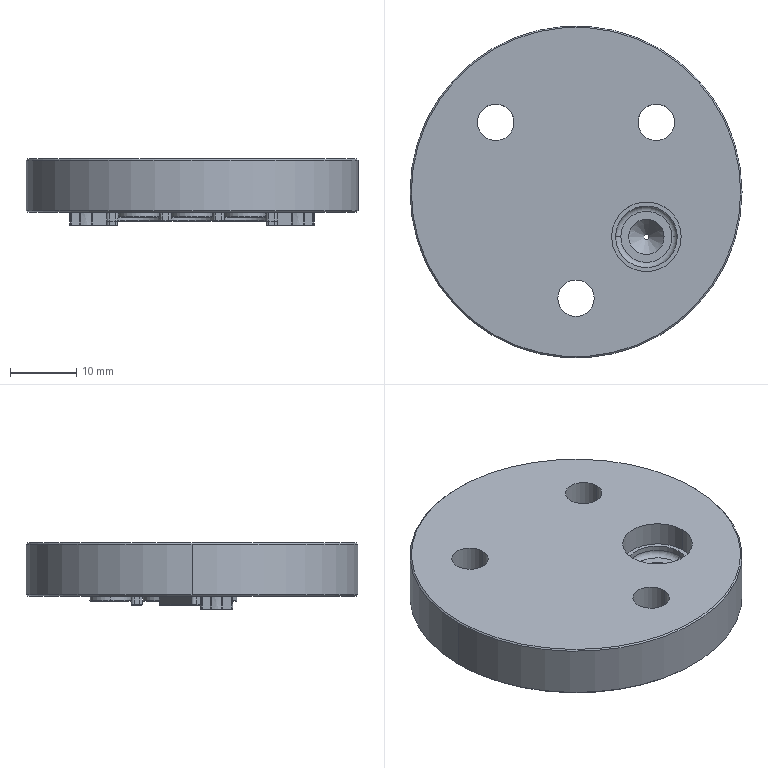Part | STEP file | Cavity | 1 solid | 372 faces | box 50 x 50 x 9.963 mm | volume 14384 mm3 | torus 130 | cone 86 | cylinder 62 | plane 56 | spline 32 | sphere 6 | commonest cylinder face diameters 0.201 x44 5.5 x6 10 x6 9.3 x2 10.5 x2 50 x2